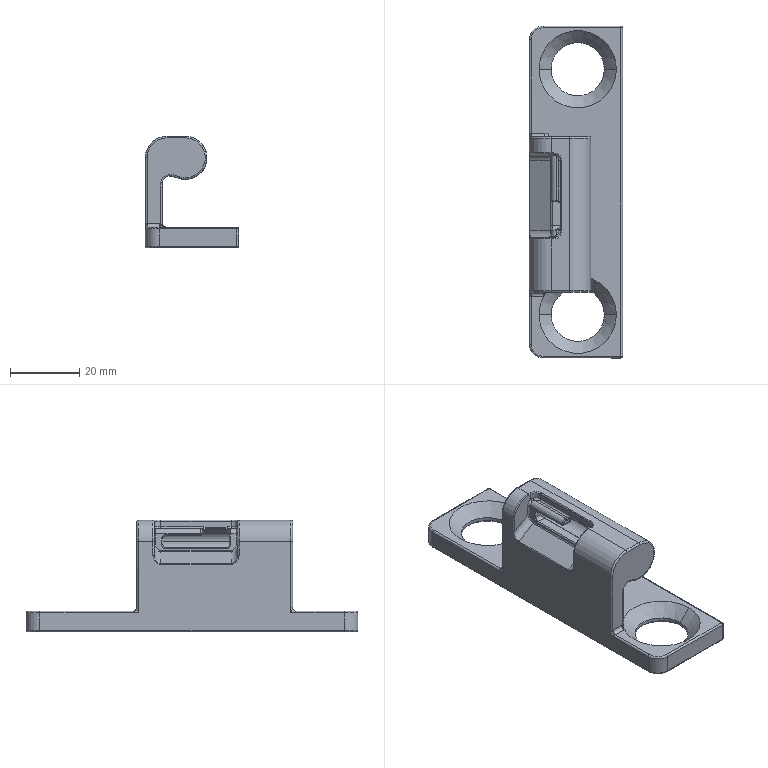Part | NX | features solid 2 | 1 solid | 186 faces | box 27 x 96.061 x 32.375 mm | volume 21063 mm3 | cylinder 70 | plane 47 | torus 32 | spline 28 | sphere 5 | cone 4 | commonest cylinder face diameters 1 x25 0.6 x13 2 x8 4 x5 15.4 x4 19 x4